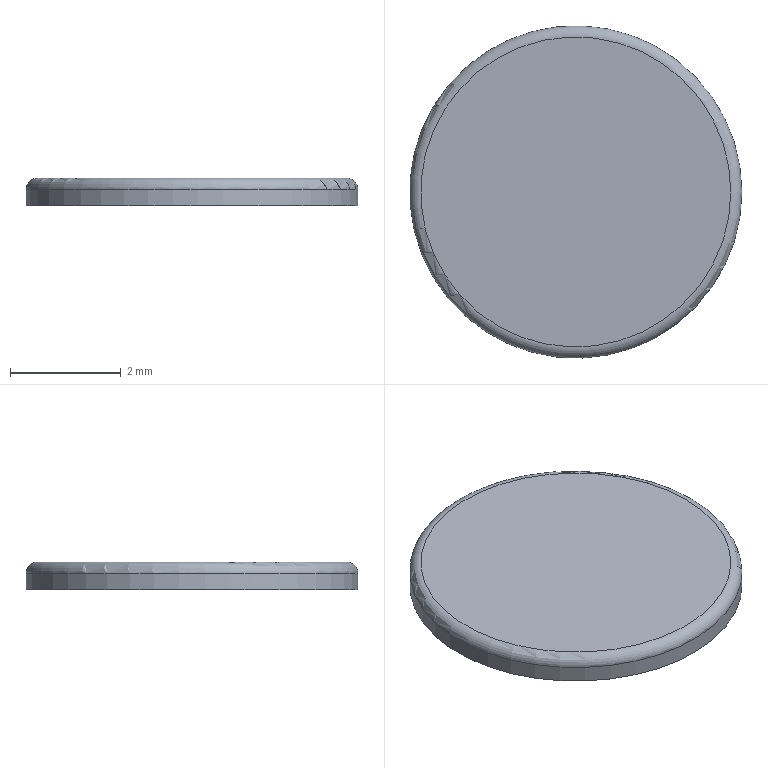Part | NX | features DATUM_CSYS 2, BLEND 1, EXTRUDE 1, SKETCH 1 | 1 solid | 4 faces | box 6 x 6 x 0.5 mm | volume 13.978 mm3 | plane 2 | cylinder 1 | torus 1 | commonest cylinder face diameters 6 x1
STEP:
#1=CARTESIAN_POINT('',(3.,0.,0.3));
#2=VERTEX_POINT('',#1);
#3=CARTESIAN_POINT('',(0.,0.,0.3));
#4=DIRECTION('',(0.,0.,1.));
#5=DIRECTION('',(1.,0.,0.));
#6=AXIS2_PLACEMENT_3D('',#3,#4,#5);
#7=CIRCLE('',#6,3.);
#8=EDGE_CURVE('',#2,#2,#7,.F.);
#9=ORIENTED_EDGE('',*,*,#8,.T.);
#10=EDGE_LOOP('',(#9));
#11=FACE_BOUND('',#10,.T.);
#12=CARTESIAN_POINT('',(3.,0.,0.));
#13=VERTEX_POINT('',#12);
#14=CARTESIAN_POINT('',(0.,0.,0.));
#15=DIRECTION('',(0.,0.,1.));
#16=DIRECTION('',(1.,0.,0.));
#17=AXIS2_PLACEMENT_3D('',#14,#15,#16);
#18=CIRCLE('',#17,3.);
#19=EDGE_CURVE('',#13,#13,#18,.T.);
#20=ORIENTED_EDGE('',*,*,#19,.T.);
#21=EDGE_LOOP('',(#20));
#22=FACE_BOUND('',#21,.T.);
#23=CARTESIAN_POINT('',(0.,0.,0.5));
#24=DIRECTION('',(0.,0.,-1.));
#25=DIRECTION('',(-1.,0.,0.));
#26=AXIS2_PLACEMENT_3D('',#23,#24,#25);
#27=CYLINDRICAL_SURFACE('',#26,3.);
#28=ADVANCED_FACE('',(#11,#22),#27,.T.);
#29=CARTESIAN_POINT('',(2.8,0.,0.5));
#30=VERTEX_POINT('',#29);
#31=CARTESIAN_POINT('',(0.,0.,0.5));
#32=DIRECTION('',(0.,0.,1.));
#33=DIRECTION('',(1.,0.,0.));
#34=AXIS2_PLACEMENT_3D('',#31,#32,#33);
#35=CIRCLE('',#34,2.8);
#36=EDGE_CURVE('',#30,#30,#35,.T.);
#37=ORIENTED_EDGE('',*,*,#36,.T.);
#38=EDGE_LOOP('',(#37));
#39=FACE_BOUND('',#38,.T.);
#40=CARTESIAN_POINT('',(0.,0.,0.5));
#41=DIRECTION('',(0.,0.,1.));
#42=DIRECTION('',(1.,0.,0.));
#43=AXIS2_PLACEMENT_3D('',#40,#41,#42);
#44=PLANE('',#43);
#45=ADVANCED_FACE('',(#39),#44,.T.);
#46=ORIENTED_EDGE('',*,*,#19,.F.);
#47=EDGE_LOOP('',(#46));
#48=FACE_BOUND('',#47,.T.);
#49=CARTESIAN_POINT('',(0.,0.,0.));
#50=DIRECTION('',(0.,0.,1.));
#51=DIRECTION('',(1.,0.,0.));
#52=AXIS2_PLACEMENT_3D('',#49,#50,#51);
#53=PLANE('',#52);
#54=ADVANCED_FACE('',(#48),#53,.F.);
#55=ORIENTED_EDGE('',*,*,#8,.F.);
#56=EDGE_LOOP('',(#55));
#57=FACE_BOUND('',#56,.T.);
#58=ORIENTED_EDGE('',*,*,#36,.F.);
#59=EDGE_LOOP('',(#58));
#60=FACE_BOUND('',#59,.T.);
#61=CARTESIAN_POINT('',(0.,0.,0.3));
#62=DIRECTION('',(0.,0.,1.));
#63=DIRECTION('',(1.,0.,0.));
#64=AXIS2_PLACEMENT_3D('',#61,#62,#63);
#65=TOROIDAL_SURFACE('',#64,2.8,0.2);
#66=ADVANCED_FACE('',(#57,#60),#65,.T.);
#67=CLOSED_SHELL('',(#28,#45,#54,#66));
#68=MANIFOLD_SOLID_BREP('',#67);
#69=(LENGTH_UNIT()NAMED_UNIT(*)SI_UNIT(.MILLI.,.METRE.));
#70=UNCERTAINTY_MEASURE_WITH_UNIT(LENGTH_MEASURE(0.00001),#69,'','');
#71=(NAMED_UNIT(*)PLANE_ANGLE_UNIT()SI_UNIT($,.RADIAN.));
#72=(NAMED_UNIT(*)SI_UNIT($,.STERADIAN.)SOLID_ANGLE_UNIT());
#73=(GEOMETRIC_REPRESENTATION_CONTEXT(3)GLOBAL_UNCERTAINTY_ASSIGNED_CONTEXT((#70))GLOBAL_UNIT_ASSIGNED_CONTEXT((#69,#71,#72))REPRESENTATION_CONTEXT('',''));
#74=ADVANCED_BREP_SHAPE_REPRESENTATION('',(#68),#73);